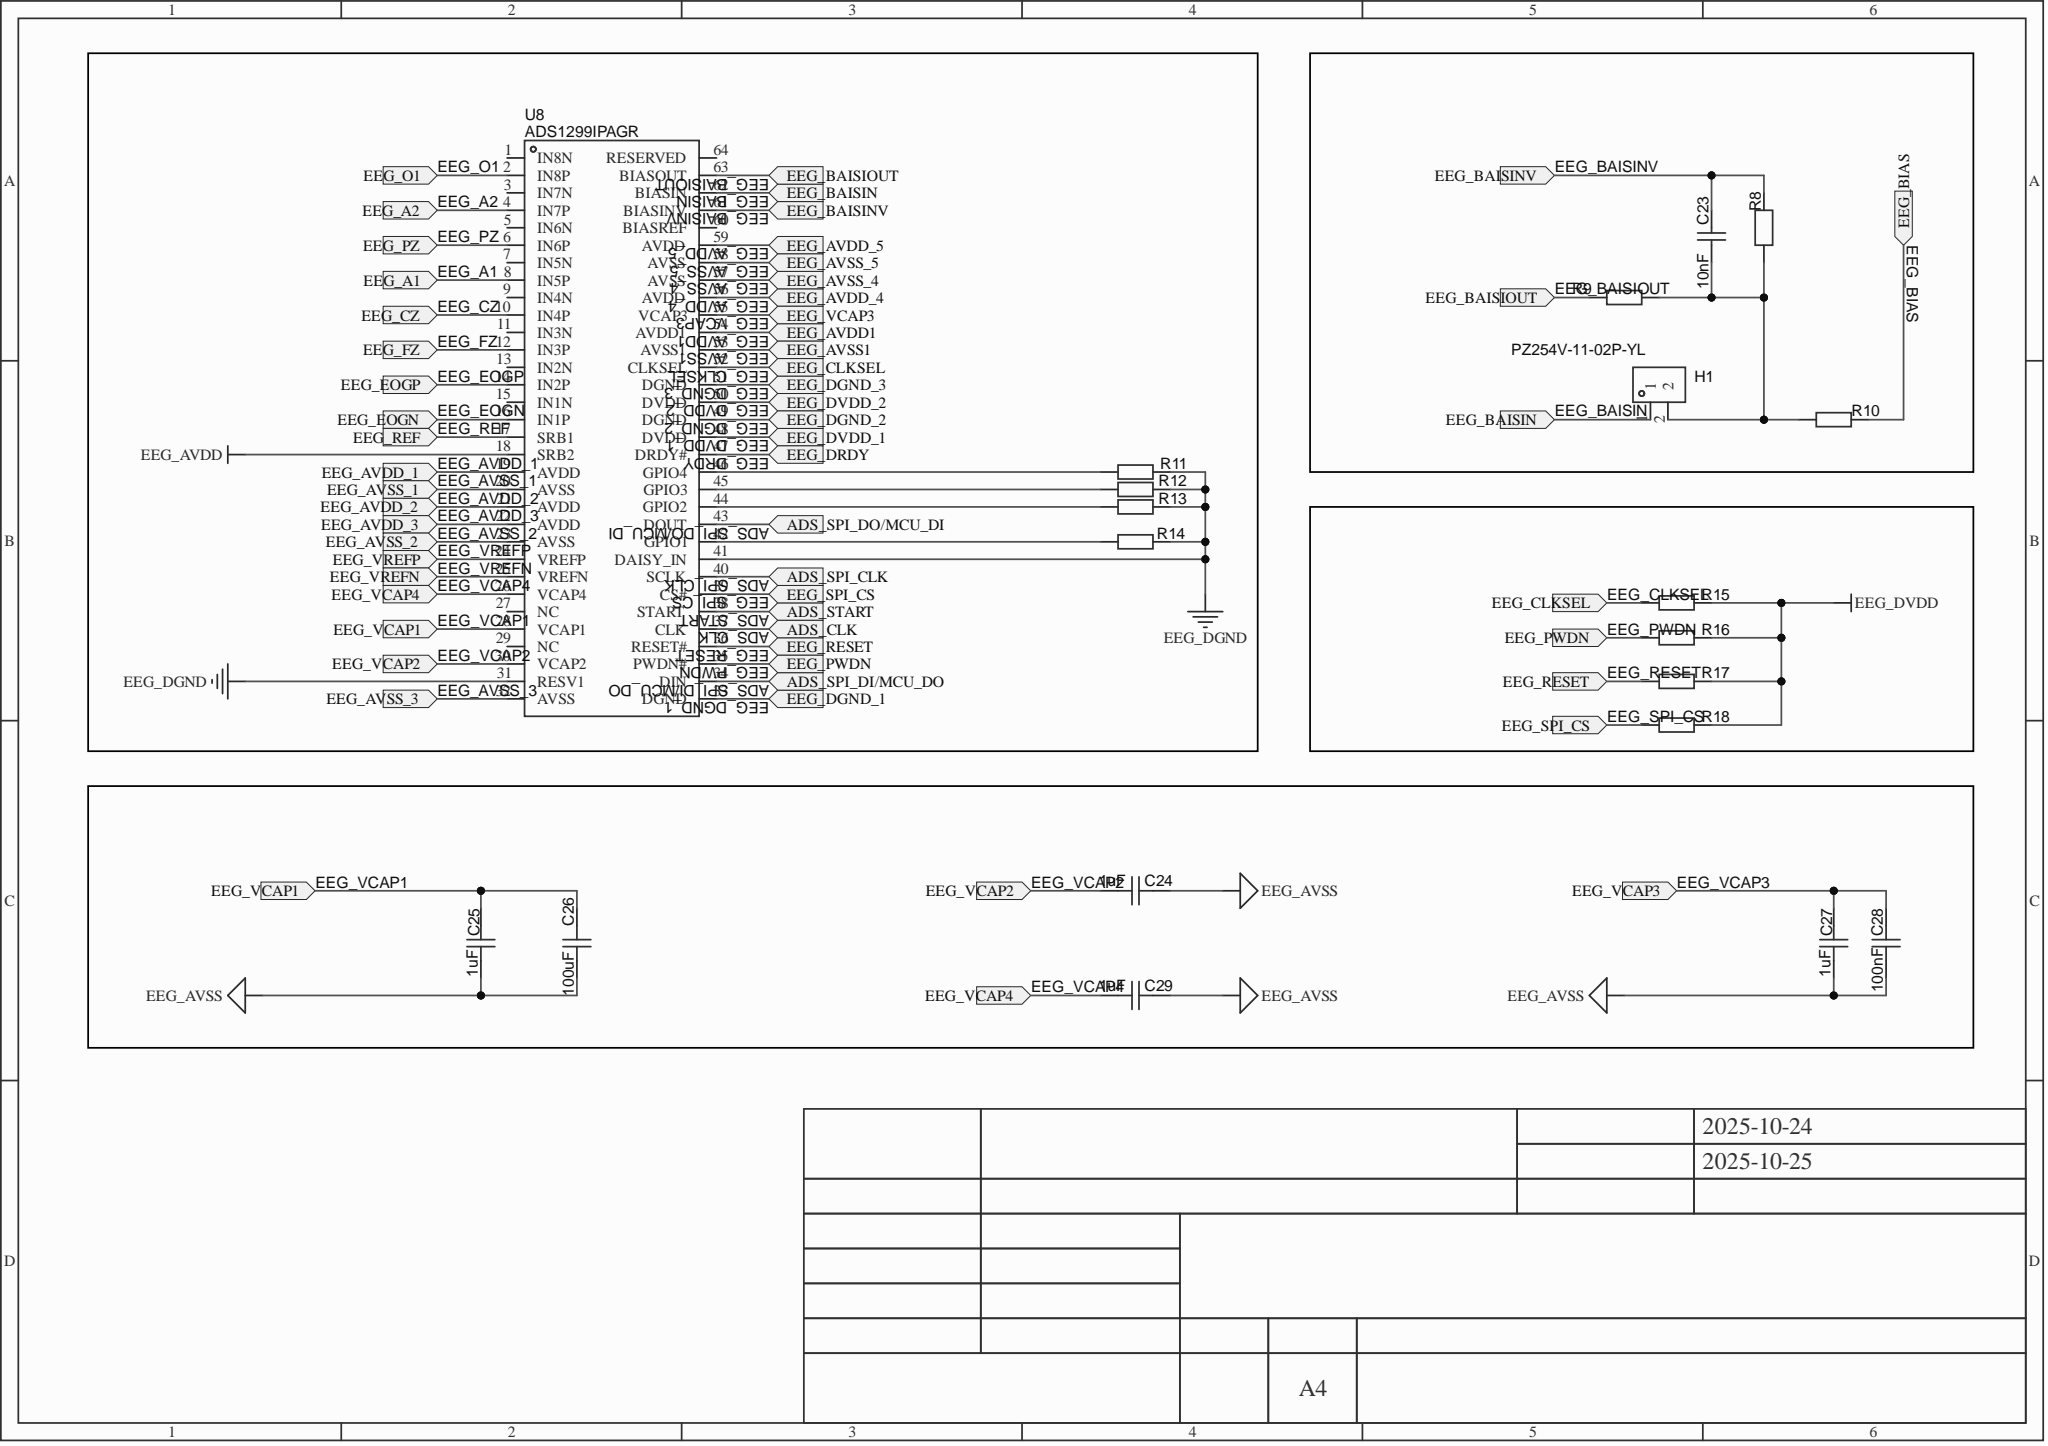Circuit board | Altium Designer | 211 parts | 126 nets | one sheet of the schematic
Parts on this sheet (reference | value | footprint):
C23 | 10nF | C0402
C24 | 1uF | C0402
C25 | 1uF | C0402
C26 | 100uF | C1206
C27 | 1uF | C0402
C28 | 100nF | C0402
C29 | 1uF | C0402
H1 | PZ254V-11-02P-YL | HDR-TH_2P-P2.54-V-M
R8 | R0402
R9 | R0402
R10 | R0402
R11 | R0402
R12 | R0402
R13 | R0402
R14 | R0402
R15 | R0402
R16 | R0402
R17 | R0402
R18 | R0402
U8 | ADS1299IPAGR | TQFP-64_L10.0-W10.0-P0.50-LS12.0-TL
Nets of these parts (net: part-pin ...):
NetR14_1: R14-1 U8-42
NetR13_1: R13-1 U8-44
NetR12_1: R12-1 U8-45
NetR11_1: R11-1 U8-46
NetC23_1: C23-1 H1-2 R8-2 R9-2 R10-1
EEG_VREFP: U8-24
EEG_VCAP4: C29-1 U8-26
EEG_VCAP3: C27-2 C28-2 U8-55
EEG_VCAP2: C24-1 U8-30
EEG_VCAP1: C25-2 C26-2 U8-28
EEG_SPI_CS: R18-1 U8-39
EEG_RESET: R17-1 U8-36
EEG_REF: U8-17
EEG_PZ: U8-6
EEG_PWDN: R16-1 U8-35
EEG_FZ: U8-12
EEG_EOGP: U8-14
EEG_EOGN: U8-16
EEG_DVDD_1: R15-2 R16-2 R17-2 R18-2 U8-48 U8-50
EEG_DRDY: U8-47
EEG_DGND_1: R11-2 R12-2 R13-2 R14-2 U8-31 U8-33 U8-41 U8-49 U8-51
EEG_CZ: U8-10
EEG_CLKSEL: R15-1 U8-52
EEG_BIAS: R10-2
EEG_BAISIOUT: R9-1 U8-63
EEG_BAISINV: C23-2 R8-1 U8-61
EEG_BAISIN: H1-1 U8-62
EEG_AVSS1: C24-2 C25-1 C26-1 C27-1 C28-1 C29-2 U8-20 U8-23 U8-25 U8-32 U8-53 U8-57 U8-58
EEG_AVDD1: U8-18 U8-19 U8-21 U8-22 U8-54 U8-56 U8-59
EEG_A1: U8-8
ADS_START: U8-38
ADS_SPI_DO/MCU_DI: U8-43
ADS_SPI_DI/MCU_DO: U8-34
ADS_SPI_CLK: U8-40
ADS_CLK: U8-37